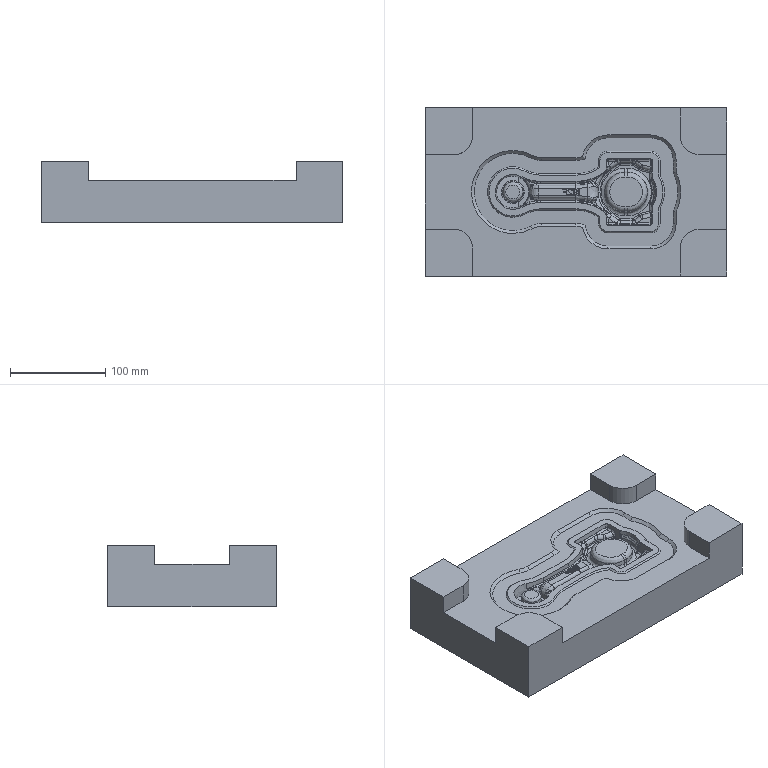CAM job | NX | 3-axis milling | part box 317 x 177 x 65 mm | stock box 317 x 177 x 65 mm
Tools:
number,name,description,diameter,corner_radius,flute_length,length,flutes
0,D30R5,Milling Tool-5 Parameters,30.0,5.0,50.0,75.0,2
0,D12,Milling Tool-5 Parameters,12.0,0.0,50.0,75.0,2
0,D6,Milling Tool-5 Parameters,6.0,0.0,50.0,75.0,2
Operations:
program,operation,operation_type,tool,method,geometry_group,spindle_rpm,surface_speed,feed_per_tooth,feed_cut,feed_plunge,cut_length_mm,path_length_mm,cut_time_min,machine_time_min
NC_PROGRAM,CAVITY_MILL,CavityMilling,D30R5,METHOD,WORKPIECE,3000.0,282.0,0.4167,2500.0,100.0,132605.839,132710.475,53.042,53.053
NC_PROGRAM,CAVITY_MILL_COPY,CavityMilling,D12,METHOD,WORKPIECE,3000.0,282.0,0.4167,2500.0,100.0,23737.202,25878.06,9.495,9.709
NC_PROGRAM,CAVITY_MILL_COPY_COPY,CavityMilling,D6,METHOD,WORKPIECE,3000.0,282.0,0.4167,2500.0,100.0,23819.393,29600.047,9.528,10.106